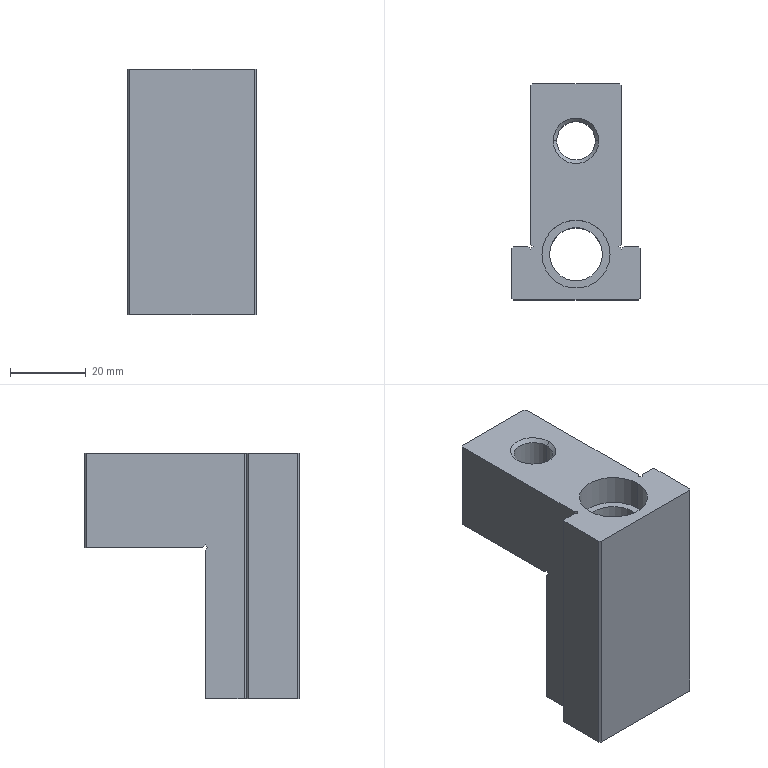Part | SolidWorks | features ICE 3, 3DProfileFeature 2, HoleWzd 2, Extrusion 1 | 1 solid | 41 faces | box 34 x 57 x 65 mm | volume 53450 mm3 | plane 29 | cylinder 8 | cone 4 | commonest cylinder face diameters 18 x4 10.2 x2 14 x2
STEP:
#1=CARTESIAN_POINT('',(-5.1,42.,64.075));
#2=VERTEX_POINT('',#1);
#3=CARTESIAN_POINT('',(5.1,42.,64.075));
#4=VERTEX_POINT('',#3);
#5=CARTESIAN_POINT('',(0.,42.,64.075));
#6=DIRECTION('',(0.,0.,1.));
#7=DIRECTION('',(1.,0.,0.));
#8=AXIS2_PLACEMENT_3D('',#5,#6,#7);
#9=CIRCLE('',#8,5.1);
#10=EDGE_CURVE('',#2,#4,#9,.T.);
#11=ORIENTED_EDGE('',*,*,#10,.F.);
#12=CARTESIAN_POINT('',(-6.025,42.,65.));
#13=VERTEX_POINT('',#12);
#14=CARTESIAN_POINT('',(-6.025,42.,65.));
#15=DIRECTION('',(-0.7071,0.,0.7071));
#16=VECTOR('',#15,1000.);
#17=LINE('',#14,#16);
#18=EDGE_CURVE('',#2,#13,#17,.T.);
#19=ORIENTED_EDGE('',*,*,#18,.T.);
#20=CARTESIAN_POINT('',(6.025,42.,65.));
#21=VERTEX_POINT('',#20);
#22=CARTESIAN_POINT('',(0.,42.,65.));
#23=DIRECTION('',(0.,0.,1.));
#24=DIRECTION('',(1.,0.,0.));
#25=AXIS2_PLACEMENT_3D('',#22,#23,#24);
#26=CIRCLE('',#25,6.025);
#27=EDGE_CURVE('',#13,#21,#26,.T.);
#28=ORIENTED_EDGE('',*,*,#27,.T.);
#29=CARTESIAN_POINT('',(6.025,42.,65.));
#30=DIRECTION('',(0.7071,0.,0.7071));
#31=VECTOR('',#30,1000.);
#32=LINE('',#29,#31);
#33=EDGE_CURVE('',#4,#21,#32,.T.);
#34=ORIENTED_EDGE('',*,*,#33,.F.);
#35=EDGE_LOOP('',(#11,#19,#28,#34));
#36=FACE_OUTER_BOUND('',#35,.T.);
#37=CARTESIAN_POINT('',(0.,42.,65.));
#38=DIRECTION('',(0.,0.,1.));
#39=DIRECTION('',(1.,0.,0.));
#40=AXIS2_PLACEMENT_3D('',#37,#38,#39);
#41=CONICAL_SURFACE('',#40,6.025,0.7854);
#42=ADVANCED_FACE('',(#36),#41,.F.);
#43=CARTESIAN_POINT('',(-5.1,42.,40.));
#44=VERTEX_POINT('',#43);
#45=CARTESIAN_POINT('',(5.1,42.,40.));
#46=VERTEX_POINT('',#45);
#47=CARTESIAN_POINT('',(0.,42.,40.));
#48=DIRECTION('',(0.,0.,1.));
#49=DIRECTION('',(0.,-1.,0.));
#50=AXIS2_PLACEMENT_3D('',#47,#48,#49);
#51=CIRCLE('',#50,5.1);
#52=EDGE_CURVE('',#44,#46,#51,.T.);
#53=ORIENTED_EDGE('',*,*,#52,.F.);
#54=CARTESIAN_POINT('',(-5.1,42.,65.));
#55=DIRECTION('',(0.,0.,1.));
#56=VECTOR('',#55,1000.);
#57=LINE('',#54,#56);
#58=EDGE_CURVE('',#44,#2,#57,.T.);
#59=ORIENTED_EDGE('',*,*,#58,.T.);
#60=ORIENTED_EDGE('',*,*,#10,.T.);
#61=CARTESIAN_POINT('',(5.1,42.,65.));
#62=DIRECTION('',(0.,0.,1.));
#63=VECTOR('',#62,1000.);
#64=LINE('',#61,#63);
#65=EDGE_CURVE('',#46,#4,#64,.T.);
#66=ORIENTED_EDGE('',*,*,#65,.F.);
#67=EDGE_LOOP('',(#53,#59,#60,#66));
#68=FACE_OUTER_BOUND('',#67,.T.);
#69=CARTESIAN_POINT('',(0.,42.,65.));
#70=DIRECTION('',(0.,0.,1.));
#71=DIRECTION('',(1.,0.,0.));
#72=AXIS2_PLACEMENT_3D('',#69,#70,#71);
#73=CYLINDRICAL_SURFACE('',#72,5.1);
#74=ADVANCED_FACE('',(#68),#73,.F.);
#75=CARTESIAN_POINT('',(7.,12.,9.025));
#76=VERTEX_POINT('',#75);
#77=CARTESIAN_POINT('',(-7.,12.,9.025));
#78=VERTEX_POINT('',#77);
#79=CARTESIAN_POINT('',(0.,12.,9.025));
#80=DIRECTION('',(0.,0.,-1.));
#81=DIRECTION('',(-1.,0.,0.));
#82=AXIS2_PLACEMENT_3D('',#79,#80,#81);
#83=CIRCLE('',#82,7.);
#84=EDGE_CURVE('',#76,#78,#83,.T.);
#85=ORIENTED_EDGE('',*,*,#84,.F.);
#86=CARTESIAN_POINT('',(8.025,12.,8.));
#87=VERTEX_POINT('',#86);
#88=CARTESIAN_POINT('',(8.025,12.,8.));
#89=DIRECTION('',(0.7071,0.,-0.7071));
#90=VECTOR('',#89,1000.);
#91=LINE('',#88,#90);
#92=EDGE_CURVE('',#76,#87,#91,.T.);
#93=ORIENTED_EDGE('',*,*,#92,.T.);
#94=CARTESIAN_POINT('',(-8.025,12.,8.));
#95=VERTEX_POINT('',#94);
#96=CARTESIAN_POINT('',(0.,12.,8.));
#97=DIRECTION('',(0.,0.,-1.));
#98=DIRECTION('',(-1.,0.,0.));
#99=AXIS2_PLACEMENT_3D('',#96,#97,#98);
#100=CIRCLE('',#99,8.025);
#101=EDGE_CURVE('',#87,#95,#100,.T.);
#102=ORIENTED_EDGE('',*,*,#101,.T.);
#103=CARTESIAN_POINT('',(-8.025,12.,8.));
#104=DIRECTION('',(-0.7071,0.,-0.7071));
#105=VECTOR('',#104,1000.);
#106=LINE('',#103,#105);
#107=EDGE_CURVE('',#78,#95,#106,.T.);
#108=ORIENTED_EDGE('',*,*,#107,.F.);
#109=EDGE_LOOP('',(#85,#93,#102,#108));
#110=FACE_OUTER_BOUND('',#109,.T.);
#111=CARTESIAN_POINT('',(0.,12.,8.));
#112=DIRECTION('',(0.,0.,-1.));
#113=DIRECTION('',(-1.,0.,0.));
#114=AXIS2_PLACEMENT_3D('',#111,#112,#113);
#115=CONICAL_SURFACE('',#114,8.025,0.7854);
#116=ADVANCED_FACE('',(#110),#115,.F.);
#117=CARTESIAN_POINT('',(-7.,12.,57.));
#118=VERTEX_POINT('',#117);
#119=CARTESIAN_POINT('',(7.,12.,57.));
#120=VERTEX_POINT('',#119);
#121=CARTESIAN_POINT('',(0.,12.,57.));
#122=DIRECTION('',(0.,0.,1.));
#123=DIRECTION('',(1.,0.,0.));
#124=AXIS2_PLACEMENT_3D('',#121,#122,#123);
#125=CIRCLE('',#124,7.);
#126=EDGE_CURVE('',#118,#120,#125,.T.);
#127=ORIENTED_EDGE('',*,*,#126,.T.);
#128=CARTESIAN_POINT('',(7.,12.,8.));
#129=DIRECTION('',(0.,0.,-1.));
#130=VECTOR('',#129,1000.);
#131=LINE('',#128,#130);
#132=EDGE_CURVE('',#120,#76,#131,.T.);
#133=ORIENTED_EDGE('',*,*,#132,.T.);
#134=ORIENTED_EDGE('',*,*,#84,.T.);
#135=CARTESIAN_POINT('',(-7.,12.,8.));
#136=DIRECTION('',(0.,0.,-1.));
#137=VECTOR('',#136,1000.);
#138=LINE('',#135,#137);
#139=EDGE_CURVE('',#118,#78,#138,.T.);
#140=ORIENTED_EDGE('',*,*,#139,.F.);
#141=EDGE_LOOP('',(#127,#133,#134,#140));
#142=FACE_OUTER_BOUND('',#141,.T.);
#143=CARTESIAN_POINT('',(0.,12.,8.));
#144=DIRECTION('',(0.,0.,-1.));
#145=DIRECTION('',(-1.,0.,0.));
#146=AXIS2_PLACEMENT_3D('',#143,#144,#145);
#147=CYLINDRICAL_SURFACE('',#146,7.);
#148=ADVANCED_FACE('',(#142),#147,.F.);
#149=CARTESIAN_POINT('',(9.,12.,8.));
#150=VERTEX_POINT('',#149);
#151=CARTESIAN_POINT('',(-9.,12.,8.));
#152=VERTEX_POINT('',#151);
#153=CARTESIAN_POINT('',(0.,12.,8.));
#154=DIRECTION('',(0.,0.,-1.));
#155=DIRECTION('',(-1.,0.,0.));
#156=AXIS2_PLACEMENT_3D('',#153,#154,#155);
#157=CIRCLE('',#156,9.);
#158=EDGE_CURVE('',#150,#152,#157,.T.);
#159=ORIENTED_EDGE('',*,*,#158,.F.);
#160=CARTESIAN_POINT('',(9.,12.,0.));
#161=VERTEX_POINT('',#160);
#162=CARTESIAN_POINT('',(9.,12.,8.));
#163=DIRECTION('',(0.,0.,-1.));
#164=VECTOR('',#163,1000.);
#165=LINE('',#162,#164);
#166=EDGE_CURVE('',#150,#161,#165,.T.);
#167=ORIENTED_EDGE('',*,*,#166,.T.);
#168=CARTESIAN_POINT('',(-9.,12.,0.));
#169=VERTEX_POINT('',#168);
#170=CARTESIAN_POINT('',(0.,12.,0.));
#171=DIRECTION('',(0.,0.,-1.));
#172=DIRECTION('',(-1.,0.,0.));
#173=AXIS2_PLACEMENT_3D('',#170,#171,#172);
#174=CIRCLE('',#173,9.);
#175=EDGE_CURVE('',#161,#169,#174,.T.);
#176=ORIENTED_EDGE('',*,*,#175,.T.);
#177=CARTESIAN_POINT('',(-9.,12.,8.));
#178=DIRECTION('',(0.,0.,-1.));
#179=VECTOR('',#178,1000.);
#180=LINE('',#177,#179);
#181=EDGE_CURVE('',#152,#169,#180,.T.);
#182=ORIENTED_EDGE('',*,*,#181,.F.);
#183=EDGE_LOOP('',(#159,#167,#176,#182));
#184=FACE_OUTER_BOUND('',#183,.T.);
#185=CARTESIAN_POINT('',(0.,12.,8.));
#186=DIRECTION('',(0.,0.,-1.));
#187=DIRECTION('',(-1.,0.,0.));
#188=AXIS2_PLACEMENT_3D('',#185,#186,#187);
#189=CYLINDRICAL_SURFACE('',#188,9.);
#190=ADVANCED_FACE('',(#184),#189,.F.);
#191=CARTESIAN_POINT('',(-9.,12.,57.));
#192=VERTEX_POINT('',#191);
#193=CARTESIAN_POINT('',(9.,12.,57.));
#194=VERTEX_POINT('',#193);
#195=CARTESIAN_POINT('',(0.,12.,57.));
#196=DIRECTION('',(0.,0.,1.));
#197=DIRECTION('',(1.,0.,0.));
#198=AXIS2_PLACEMENT_3D('',#195,#196,#197);
#199=CIRCLE('',#198,9.);
#200=EDGE_CURVE('',#192,#194,#199,.T.);
#201=ORIENTED_EDGE('',*,*,#200,.F.);
#202=CARTESIAN_POINT('',(-9.,12.,65.));
#203=VERTEX_POINT('',#202);
#204=CARTESIAN_POINT('',(-9.,12.,57.));
#205=DIRECTION('',(0.,0.,1.));
#206=VECTOR('',#205,1000.);
#207=LINE('',#204,#206);
#208=EDGE_CURVE('',#192,#203,#207,.T.);
#209=ORIENTED_EDGE('',*,*,#208,.T.);
#210=CARTESIAN_POINT('',(9.,12.,65.));
#211=VERTEX_POINT('',#210);
#212=CARTESIAN_POINT('',(0.,12.,65.));
#213=DIRECTION('',(0.,0.,1.));
#214=DIRECTION('',(1.,0.,0.));
#215=AXIS2_PLACEMENT_3D('',#212,#213,#214);
#216=CIRCLE('',#215,9.);
#217=EDGE_CURVE('',#203,#211,#216,.T.);
#218=ORIENTED_EDGE('',*,*,#217,.T.);
#219=CARTESIAN_POINT('',(9.,12.,57.));
#220=DIRECTION('',(0.,0.,1.));
#221=VECTOR('',#220,1000.);
#222=LINE('',#219,#221);
#223=EDGE_CURVE('',#194,#211,#222,.T.);
#224=ORIENTED_EDGE('',*,*,#223,.F.);
#225=EDGE_LOOP('',(#201,#209,#218,#224));
#226=FACE_OUTER_BOUND('',#225,.T.);
#227=CARTESIAN_POINT('',(0.,12.,57.));
#228=DIRECTION('',(0.,0.,1.));
#229=DIRECTION('',(1.,0.,0.));
#230=AXIS2_PLACEMENT_3D('',#227,#228,#229);
#231=CYLINDRICAL_SURFACE('',#230,9.);
#232=ADVANCED_FACE('',(#226),#231,.F.);
#233=CARTESIAN_POINT('',(-11.5,57.,65.));
#234=VERTEX_POINT('',#233);
#235=CARTESIAN_POINT('',(-11.5,57.,40.));
#236=VERTEX_POINT('',#235);
#237=CARTESIAN_POINT('',(-11.5,57.,65.));
#238=DIRECTION('',(0.,0.,-1.));
#239=VECTOR('',#238,1000.);
#240=LINE('',#237,#239);
#241=EDGE_CURVE('',#234,#236,#240,.T.);
#242=ORIENTED_EDGE('',*,*,#241,.T.);
#243=CARTESIAN_POINT('',(-12.,56.5,40.));
#244=VERTEX_POINT('',#243);
#245=CARTESIAN_POINT('',(-12.,56.5,40.));
#246=DIRECTION('',(-0.7071,-0.7071,0.));
#247=VECTOR('',#246,1000.);
#248=LINE('',#245,#247);
#249=EDGE_CURVE('',#236,#244,#248,.T.);
#250=ORIENTED_EDGE('',*,*,#249,.T.);
#251=CARTESIAN_POINT('',(-12.,56.5,65.));
#252=VERTEX_POINT('',#251);
#253=CARTESIAN_POINT('',(-12.,56.5,65.));
#254=DIRECTION('',(0.,0.,-1.));
#255=VECTOR('',#254,1000.);
#256=LINE('',#253,#255);
#257=EDGE_CURVE('',#252,#244,#256,.T.);
#258=ORIENTED_EDGE('',*,*,#257,.F.);
#259=CARTESIAN_POINT('',(-12.,56.5,65.));
#260=DIRECTION('',(-0.7071,-0.7071,0.));
#261=VECTOR('',#260,1000.);
#262=LINE('',#259,#261);
#263=EDGE_CURVE('',#234,#252,#262,.T.);
#264=ORIENTED_EDGE('',*,*,#263,.F.);
#265=EDGE_LOOP('',(#242,#250,#258,#264));
#266=FACE_OUTER_BOUND('',#265,.T.);
#267=CARTESIAN_POINT('',(-12.,56.5,65.));
#268=DIRECTION('',(0.7071,-0.7071,0.));
#269=DIRECTION('',(0.7071,0.7071,0.));
#270=AXIS2_PLACEMENT_3D('',#267,#268,#269);
#271=PLANE('',#270);
#272=ADVANCED_FACE('',(#266),#271,.F.);
#273=ORIENTED_EDGE('',*,*,#257,.T.);
#274=CARTESIAN_POINT('',(-12.,25.707,40.));
#275=VERTEX_POINT('',#274);
#276=CARTESIAN_POINT('',(-12.,14.707,40.));
#277=DIRECTION('',(0.,-1.,0.));
#278=VECTOR('',#277,1000.);
#279=LINE('',#276,#278);
#280=EDGE_CURVE('',#244,#275,#279,.T.);
#281=ORIENTED_EDGE('',*,*,#280,.T.);
#282=CARTESIAN_POINT('',(-12.,25.,40.707));
#283=VERTEX_POINT('',#282);
#284=CARTESIAN_POINT('',(-12.,7.707,58.));
#285=DIRECTION('',(0.,-0.7071,0.7071));
#286=VECTOR('',#285,1000.);
#287=LINE('',#284,#286);
#288=EDGE_CURVE('',#275,#283,#287,.T.);
#289=ORIENTED_EDGE('',*,*,#288,.T.);
#290=CARTESIAN_POINT('',(-12.,24.293,40.));
#291=VERTEX_POINT('',#290);
#292=CARTESIAN_POINT('',(-12.,32.,47.707));
#293=DIRECTION('',(0.,-0.7071,-0.7071));
#294=VECTOR('',#293,1000.);
#295=LINE('',#292,#294);
#296=EDGE_CURVE('',#283,#291,#295,.T.);
#297=ORIENTED_EDGE('',*,*,#296,.T.);
#298=CARTESIAN_POINT('',(-12.,25.,39.293));
#299=VERTEX_POINT('',#298);
#300=CARTESIAN_POINT('',(-12.,7.,57.293));
#301=DIRECTION('',(0.,0.7071,-0.7071));
#302=VECTOR('',#301,1000.);
#303=LINE('',#300,#302);
#304=EDGE_CURVE('',#291,#299,#303,.T.);
#305=ORIENTED_EDGE('',*,*,#304,.T.);
#306=CARTESIAN_POINT('',(-12.,25.,0.));
#307=VERTEX_POINT('',#306);
#308=CARTESIAN_POINT('',(-12.,25.,65.));
#309=DIRECTION('',(0.,0.,-1.));
#310=VECTOR('',#309,1000.);
#311=LINE('',#308,#310);
#312=EDGE_CURVE('',#299,#307,#311,.T.);
#313=ORIENTED_EDGE('',*,*,#312,.T.);
#314=CARTESIAN_POINT('',(-12.,14.707,0.));
#315=VERTEX_POINT('',#314);
#316=CARTESIAN_POINT('',(-12.,14.707,0.));
#317=DIRECTION('',(0.,-1.,0.));
#318=VECTOR('',#317,1000.);
#319=LINE('',#316,#318);
#320=EDGE_CURVE('',#307,#315,#319,.T.);
#321=ORIENTED_EDGE('',*,*,#320,.T.);
#322=CARTESIAN_POINT('',(-12.,14.707,65.));
#323=VERTEX_POINT('',#322);
#324=CARTESIAN_POINT('',(-12.,14.707,65.));
#325=DIRECTION('',(0.,0.,-1.));
#326=VECTOR('',#325,1000.);
#327=LINE('',#324,#326);
#328=EDGE_CURVE('',#323,#315,#327,.T.);
#329=ORIENTED_EDGE('',*,*,#328,.F.);
#330=CARTESIAN_POINT('',(-12.,14.707,65.));
#331=DIRECTION('',(0.,-1.,0.));
#332=VECTOR('',#331,1000.);
#333=LINE('',#330,#332);
#334=EDGE_CURVE('',#252,#323,#333,.T.);
#335=ORIENTED_EDGE('',*,*,#334,.F.);
#336=EDGE_LOOP('',(#273,#281,#289,#297,#305,#313,#321,#329,#335));
#337=FACE_OUTER_BOUND('',#336,.T.);
#338=CARTESIAN_POINT('',(-12.,14.707,65.));
#339=DIRECTION('',(1.,0.,0.));
#340=DIRECTION('',(0.,0.,-1.));
#341=AXIS2_PLACEMENT_3D('',#338,#339,#340);
#342=PLANE('',#341);
#343=ADVANCED_FACE('',(#337),#342,.F.);
#344=CARTESIAN_POINT('',(-11.293,14.,0.));
#345=VERTEX_POINT('',#344);
#346=CARTESIAN_POINT('',(-12.,14.707,0.));
#347=DIRECTION('',(0.7071,-0.7071,0.));
#348=VECTOR('',#347,1000.);
#349=LINE('',#346,#348);
#350=EDGE_CURVE('',#315,#345,#349,.T.);
#351=ORIENTED_EDGE('',*,*,#350,.T.);
#352=CARTESIAN_POINT('',(-11.293,14.,65.));
#353=VERTEX_POINT('',#352);
#354=CARTESIAN_POINT('',(-11.293,14.,65.));
#355=DIRECTION('',(0.,0.,-1.));
#356=VECTOR('',#355,1000.);
#357=LINE('',#354,#356);
#358=EDGE_CURVE('',#353,#345,#357,.T.);
#359=ORIENTED_EDGE('',*,*,#358,.F.);
#360=CARTESIAN_POINT('',(-12.,14.707,65.));
#361=DIRECTION('',(0.7071,-0.7071,0.));
#362=VECTOR('',#361,1000.);
#363=LINE('',#360,#362);
#364=EDGE_CURVE('',#323,#353,#363,.T.);
#365=ORIENTED_EDGE('',*,*,#364,.F.);
#366=ORIENTED_EDGE('',*,*,#328,.T.);
#367=EDGE_LOOP('',(#351,#359,#365,#366));
#368=FACE_OUTER_BOUND('',#367,.T.);
#369=CARTESIAN_POINT('',(-12.,14.707,65.));
#370=DIRECTION('',(0.7071,0.7071,0.));
#371=DIRECTION('',(-0.7071,0.7071,0.));
#372=AXIS2_PLACEMENT_3D('',#369,#370,#371);
#373=PLANE('',#372);
#374=ADVANCED_FACE('',(#368),#373,.F.);
#375=CARTESIAN_POINT('',(-12.,13.293,0.));
#376=VERTEX_POINT('',#375);
#377=CARTESIAN_POINT('',(-12.,13.293,0.));
#378=DIRECTION('',(-0.7071,-0.7071,0.));
#379=VECTOR('',#378,1000.);
#380=LINE('',#377,#379);
#381=EDGE_CURVE('',#345,#376,#380,.T.);
#382=ORIENTED_EDGE('',*,*,#381,.T.);
#383=CARTESIAN_POINT('',(-12.,13.293,65.));
#384=VERTEX_POINT('',#383);
#385=CARTESIAN_POINT('',(-12.,13.293,65.));
#386=DIRECTION('',(0.,0.,-1.));
#387=VECTOR('',#386,1000.);
#388=LINE('',#385,#387);
#389=EDGE_CURVE('',#384,#376,#388,.T.);
#390=ORIENTED_EDGE('',*,*,#389,.F.);
#391=CARTESIAN_POINT('',(-12.,13.293,65.));
#392=DIRECTION('',(-0.7071,-0.7071,0.));
#393=VECTOR('',#392,1000.);
#394=LINE('',#391,#393);
#395=EDGE_CURVE('',#353,#384,#394,.T.);
#396=ORIENTED_EDGE('',*,*,#395,.F.);
#397=ORIENTED_EDGE('',*,*,#358,.T.);
#398=EDGE_LOOP('',(#382,#390,#396,#397));
#399=FACE_OUTER_BOUND('',#398,.T.);
#400=CARTESIAN_POINT('',(-12.,13.293,65.));
#401=DIRECTION('',(0.7071,-0.7071,0.));
#402=DIRECTION('',(0.7071,0.7071,0.));
#403=AXIS2_PLACEMENT_3D('',#400,#401,#402);
#404=PLANE('',#403);
#405=ADVANCED_FACE('',(#399),#404,.F.);
#406=CARTESIAN_POINT('',(-12.707,14.,0.));
#407=VERTEX_POINT('',#406);
#408=CARTESIAN_POINT('',(-12.707,14.,0.));
#409=DIRECTION('',(-0.7071,0.7071,0.));
#410=VECTOR('',#409,1000.);
#411=LINE('',#408,#410);
#412=EDGE_CURVE('',#376,#407,#411,.T.);
#413=ORIENTED_EDGE('',*,*,#412,.T.);
#414=CARTESIAN_POINT('',(-12.707,14.,65.));
#415=VERTEX_POINT('',#414);
#416=CARTESIAN_POINT('',(-12.707,14.,65.));
#417=DIRECTION('',(0.,0.,-1.));
#418=VECTOR('',#417,1000.);
#419=LINE('',#416,#418);
#420=EDGE_CURVE('',#415,#407,#419,.T.);
#421=ORIENTED_EDGE('',*,*,#420,.F.);
#422=CARTESIAN_POINT('',(-12.707,14.,65.));
#423=DIRECTION('',(-0.7071,0.7071,0.));
#424=VECTOR('',#423,1000.);
#425=LINE('',#422,#424);
#426=EDGE_CURVE('',#384,#415,#425,.T.);
#427=ORIENTED_EDGE('',*,*,#426,.F.);
#428=ORIENTED_EDGE('',*,*,#389,.T.);
#429=EDGE_LOOP('',(#413,#421,#427,#428));
#430=FACE_OUTER_BOUND('',#429,.T.);
#431=CARTESIAN_POINT('',(-12.707,14.,65.));
#432=DIRECTION('',(-0.7071,-0.7071,0.));
#433=DIRECTION('',(0.7071,-0.7071,0.));
#434=AXIS2_PLACEMENT_3D('',#431,#432,#433);
#435=PLANE('',#434);
#436=ADVANCED_FACE('',(#430),#435,.F.);
#437=CARTESIAN_POINT('',(-16.5,14.,0.));
#438=VERTEX_POINT('',#437);
#439=CARTESIAN_POINT('',(-16.5,14.,0.));
#440=DIRECTION('',(-1.,0.,0.));
#441=VECTOR('',#440,1000.);
#442=LINE('',#439,#441);
#443=EDGE_CURVE('',#407,#438,#442,.T.);
#444=ORIENTED_EDGE('',*,*,#443,.T.);
#445=CARTESIAN_POINT('',(-16.5,14.,65.));
#446=VERTEX_POINT('',#445);
#447=CARTESIAN_POINT('',(-16.5,14.,65.));
#448=DIRECTION('',(0.,0.,-1.));
#449=VECTOR('',#448,1000.);
#450=LINE('',#447,#449);
#451=EDGE_CURVE('',#446,#438,#450,.T.);
#452=ORIENTED_EDGE('',*,*,#451,.F.);
#453=CARTESIAN_POINT('',(-16.5,14.,65.));
#454=DIRECTION('',(-1.,0.,0.));
#455=VECTOR('',#454,1000.);
#456=LINE('',#453,#455);
#457=EDGE_CURVE('',#415,#446,#456,.T.);
#458=ORIENTED_EDGE('',*,*,#457,.F.);
#459=ORIENTED_EDGE('',*,*,#420,.T.);
#460=EDGE_LOOP('',(#444,#452,#458,#459));
#461=FACE_OUTER_BOUND('',#460,.T.);
#462=CARTESIAN_POINT('',(-16.5,14.,65.));
#463=DIRECTION('',(0.,-1.,0.));
#464=DIRECTION('',(1.,0.,0.));
#465=AXIS2_PLACEMENT_3D('',#462,#463,#464);
#466=PLANE('',#465);
#467=ADVANCED_FACE('',(#461),#466,.F.);
#468=CARTESIAN_POINT('',(-17.,13.5,0.));
#469=VERTEX_POINT('',#468);
#470=CARTESIAN_POINT('',(-17.,13.5,0.));
#471=DIRECTION('',(-0.7071,-0.7071,0.));
#472=VECTOR('',#471,1000.);
#473=LINE('',#470,#472);
#474=EDGE_CURVE('',#438,#469,#473,.T.);
#475=ORIENTED_EDGE('',*,*,#474,.T.);
#476=CARTESIAN_POINT('',(-17.,13.5,65.));
#477=VERTEX_POINT('',#476);
#478=CARTESIAN_POINT('',(-17.,13.5,65.));
#479=DIRECTION('',(0.,0.,-1.));
#480=VECTOR('',#479,1000.);
#481=LINE('',#478,#480);
#482=EDGE_CURVE('',#477,#469,#481,.T.);
#483=ORIENTED_EDGE('',*,*,#482,.F.);
#484=CARTESIAN_POINT('',(-17.,13.5,65.));
#485=DIRECTION('',(-0.7071,-0.7071,0.));
#486=VECTOR('',#485,1000.);
#487=LINE('',#484,#486);
#488=EDGE_CURVE('',#446,#477,#487,.T.);
#489=ORIENTED_EDGE('',*,*,#488,.F.);
#490=ORIENTED_EDGE('',*,*,#451,.T.);
#491=EDGE_LOOP('',(#475,#483,#489,#490));
#492=FACE_OUTER_BOUND('',#491,.T.);
#493=CARTESIAN_POINT('',(-17.,13.5,65.));
#494=DIRECTION('',(0.7071,-0.7071,0.));
#495=DIRECTION('',(0.7071,0.7071,0.));
#496=AXIS2_PLACEMENT_3D('',#493,#494,#495);
#497=PLANE('',#496);
#498=ADVANCED_FACE('',(#492),#497,.F.);
#499=CARTESIAN_POINT('',(-17.,0.5,0.));
#500=VERTEX_POINT('',#499);
#501=CARTESIAN_POINT('',(-17.,0.5,0.));
#502=DIRECTION('',(0.,-1.,0.));
#503=VECTOR('',#502,1000.);
#504=LINE('',#501,#503);
#505=EDGE_CURVE('',#469,#500,#504,.T.);
#506=ORIENTED_EDGE('',*,*,#505,.T.);
#507=CARTESIAN_POINT('',(-17.,0.5,65.));
#508=VERTEX_POINT('',#507);
#509=CARTESIAN_POINT('',(-17.,0.5,65.));
#510=DIRECTION('',(0.,0.,-1.));
#511=VECTOR('',#510,1000.);
#512=LINE('',#509,#511);
#513=EDGE_CURVE('',#508,#500,#512,.T.);
#514=ORIENTED_EDGE('',*,*,#513,.F.);
#515=CARTESIAN_POINT('',(-17.,0.5,65.));
#516=DIRECTION('',(0.,-1.,0.));
#517=VECTOR('',#516,1000.);
#518=LINE('',#515,#517);
#519=EDGE_CURVE('',#477,#508,#518,.T.);
#520=ORIENTED_EDGE('',*,*,#519,.F.);
#521=ORIENTED_EDGE('',*,*,#482,.T.);
#522=EDGE_LOOP('',(#506,#514,#520,#521));
#523=FACE_OUTER_BOUND('',#522,.T.);
#524=CARTESIAN_POINT('',(-17.,0.5,65.));
#525=DIRECTION('',(1.,0.,0.));
#526=DIRECTION('',(0.,0.,-1.));
#527=AXIS2_PLACEMENT_3D('',#524,#525,#526);
#528=PLANE('',#527);
#529=ADVANCED_FACE('',(#523),#528,.F.);
#530=CARTESIAN_POINT('',(-16.5,0.,0.));
#531=VERTEX_POINT('',#530);
#532=CARTESIAN_POINT('',(-16.5,0.,0.));
#533=DIRECTION('',(0.7071,-0.7071,0.));
#534=VECTOR('',#533,1000.);
#535=LINE('',#532,#534);
#536=EDGE_CURVE('',#500,#531,#535,.T.);
#537=ORIENTED_EDGE('',*,*,#536,.T.);
#538=CARTESIAN_POINT('',(-16.5,0.,65.));
#539=VERTEX_POINT('',#538);
#540=CARTESIAN_POINT('',(-16.5,0.,65.));
#541=DIRECTION('',(0.,0.,-1.));
#542=VECTOR('',#541,1000.);
#543=LINE('',#540,#542);
#544=EDGE_CURVE('',#539,#531,#543,.T.);
#545=ORIENTED_EDGE('',*,*,#544,.F.);
#546=CARTESIAN_POINT('',(-16.5,0.,65.));
#547=DIRECTION('',(0.7071,-0.7071,0.));
#548=VECTOR('',#547,1000.);
#549=LINE('',#546,#548);
#550=EDGE_CURVE('',#508,#539,#549,.T.);
#551=ORIENTED_EDGE('',*,*,#550,.F.);
#552=ORIENTED_EDGE('',*,*,#513,.T.);
#553=EDGE_LOOP('',(#537,#545,#551,#552));
#554=FACE_OUTER_BOUND('',#553,.T.);
#555=CARTESIAN_POINT('',(-16.5,0.,65.));
#556=DIRECTION('',(0.7071,0.7071,0.));
#557=DIRECTION('',(-0.7071,0.7071,0.));
#558=AXIS2_PLACEMENT_3D('',#555,#556,#557);
#559=PLANE('',#558);
#560=ADVANCED_FACE('',(#554),#559,.F.);
#561=CARTESIAN_POINT('',(16.5,0.,0.));
#562=VERTEX_POINT('',#561);
#563=CARTESIAN_POINT('',(16.5,0.,0.));
#564=DIRECTION('',(1.,0.,0.));
#565=VECTOR('',#564,1000.);
#566=LINE('',#563,#565);
#567=EDGE_CURVE('',#531,#562,#566,.T.);
#568=ORIENTED_EDGE('',*,*,#567,.T.);
#569=CARTESIAN_POINT('',(16.5,0.,65.));
#570=VERTEX_POINT('',#569);
#571=CARTESIAN_POINT('',(16.5,0.,65.));
#572=DIRECTION('',(0.,0.,-1.));
#573=VECTOR('',#572,1000.);
#574=LINE('',#571,#573);
#575=EDGE_CURVE('',#570,#562,#574,.T.);
#576=ORIENTED_EDGE('',*,*,#575,.F.);
#577=CARTESIAN_POINT('',(16.5,0.,65.));
#578=DIRECTION('',(1.,0.,0.));
#579=VECTOR('',#578,1000.);
#580=LINE('',#577,#579);
#581=EDGE_CURVE('',#539,#570,#580,.T.);
#582=ORIENTED_EDGE('',*,*,#581,.F.);
#583=ORIENTED_EDGE('',*,*,#544,.T.);
#584=EDGE_LOOP('',(#568,#576,#582,#583));
#585=FACE_OUTER_BOUND('',#584,.T.);
#586=CARTESIAN_POINT('',(16.5,0.,65.));
#587=DIRECTION('',(0.,1.,0.));
#588=DIRECTION('',(0.,0.,1.));
#589=AXIS2_PLACEMENT_3D('',#586,#587,#588);
#590=PLANE('',#589);
#591=ADVANCED_FACE('',(#585),#590,.F.);
#592=CARTESIAN_POINT('',(17.,0.5,0.));
#593=VERTEX_POINT('',#592);
#594=CARTESIAN_POINT('',(16.5,0.,0.));
#595=DIRECTION('',(0.7071,0.7071,0.));
#596=VECTOR('',#595,1000.);
#597=LINE('',#594,#596);
#598=EDGE_CURVE('',#562,#593,#597,.T.);
#599=ORIENTED_EDGE('',*,*,#598,.T.);
#600=CARTESIAN_POINT('',(17.,0.5,65.));
#601=VERTEX_POINT('',#600);
#602=CARTESIAN_POINT('',(17.,0.5,65.));
#603=DIRECTION('',(0.,0.,-1.));
#604=VECTOR('',#603,1000.);
#605=LINE('',#602,#604);
#606=EDGE_CURVE('',#601,#593,#605,.T.);
#607=ORIENTED_EDGE('',*,*,#606,.F.);
#608=CARTESIAN_POINT('',(16.5,0.,65.));
#609=DIRECTION('',(0.7071,0.7071,0.));
#610=VECTOR('',#609,1000.);
#611=LINE('',#608,#610);
#612=EDGE_CURVE('',#570,#601,#611,.T.);
#613=ORIENTED_EDGE('',*,*,#612,.F.);
#614=ORIENTED_EDGE('',*,*,#575,.T.);
#615=EDGE_LOOP('',(#599,#607,#613,#614));
#616=FACE_OUTER_BOUND('',#615,.T.);
#617=CARTESIAN_POINT('',(16.5,0.,65.));
#618=DIRECTION('',(-0.7071,0.7071,0.));
#619=DIRECTION('',(-0.7071,-0.7071,0.));
#620=AXIS2_PLACEMENT_3D('',#617,#618,#619);
#621=PLANE('',#620);
#622=ADVANCED_FACE('',(#616),#621,.F.);
#623=CARTESIAN_POINT('',(17.,13.5,0.));
#624=VERTEX_POINT('',#623);
#625=CARTESIAN_POINT('',(17.,0.5,0.));
#626=DIRECTION('',(0.,1.,0.));
#627=VECTOR('',#626,1000.);
#628=LINE('',#625,#627);
#629=EDGE_CURVE('',#593,#624,#628,.T.);
#630=ORIENTED_EDGE('',*,*,#629,.T.);
#631=CARTESIAN_POINT('',(17.,13.5,65.));
#632=VERTEX_POINT('',#631);
#633=CARTESIAN_POINT('',(17.,13.5,65.));
#634=DIRECTION('',(0.,0.,-1.));
#635=VECTOR('',#634,1000.);
#636=LINE('',#633,#635);
#637=EDGE_CURVE('',#632,#624,#636,.T.);
#638=ORIENTED_EDGE('',*,*,#637,.F.);
#639=CARTESIAN_POINT('',(17.,0.5,65.));
#640=DIRECTION('',(0.,1.,0.));
#641=VECTOR('',#640,1000.);
#642=LINE('',#639,#641);
#643=EDGE_CURVE('',#601,#632,#642,.T.);
#644=ORIENTED_EDGE('',*,*,#643,.F.);
#645=ORIENTED_EDGE('',*,*,#606,.T.);
#646=EDGE_LOOP('',(#630,#638,#644,#645));
#647=FACE_OUTER_BOUND('',#646,.T.);
#648=CARTESIAN_POINT('',(17.,0.5,65.));
#649=DIRECTION('',(-1.,0.,0.));
#650=DIRECTION('',(0.,0.,1.));
#651=AXIS2_PLACEMENT_3D('',#648,#649,#650);
#652=PLANE('',#651);
#653=ADVANCED_FACE('',(#647),#652,.F.);
#654=CARTESIAN_POINT('',(16.5,14.,0.));
#655=VERTEX_POINT('',#654);
#656=CARTESIAN_POINT('',(17.,13.5,0.));
#657=DIRECTION('',(-0.7071,0.7071,0.));
#658=VECTOR('',#657,1000.);
#659=LINE('',#656,#658);
#660=EDGE_CURVE('',#624,#655,#659,.T.);
#661=ORIENTED_EDGE('',*,*,#660,.T.);
#662=CARTESIAN_POINT('',(16.5,14.,65.));
#663=VERTEX_POINT('',#662);
#664=CARTESIAN_POINT('',(16.5,14.,65.));
#665=DIRECTION('',(0.,0.,-1.));
#666=VECTOR('',#665,1000.);
#667=LINE('',#664,#666);
#668=EDGE_CURVE('',#663,#655,#667,.T.);
#669=ORIENTED_EDGE('',*,*,#668,.F.);
#670=CARTESIAN_POINT('',(17.,13.5,65.));
#671=DIRECTION('',(-0.7071,0.7071,0.));
#672=VECTOR('',#671,1000.);
#673=LINE('',#670,#672);
#674=EDGE_CURVE('',#632,#663,#673,.T.);
#675=ORIENTED_EDGE('',*,*,#674,.F.);
#676=ORIENTED_EDGE('',*,*,#637,.T.);
#677=EDGE_LOOP('',(#661,#669,#675,#676));
#678=FACE_OUTER_BOUND('',#677,.T.);
#679=CARTESIAN_POINT('',(17.,13.5,65.));
#680=DIRECTION('',(-0.7071,-0.7071,0.));
#681=DIRECTION('',(0.7071,-0.7071,0.));
#682=AXIS2_PLACEMENT_3D('',#679,#680,#681);
#683=PLANE('',#682);
#684=ADVANCED_FACE('',(#678),#683,.F.);
#685=CARTESIAN_POINT('',(12.707,14.,0.));
#686=VERTEX_POINT('',#685);
#687=CARTESIAN_POINT('',(16.5,14.,0.));
#688=DIRECTION('',(-1.,0.,0.));
#689=VECTOR('',#688,1000.);
#690=LINE('',#687,#689);
#691=EDGE_CURVE('',#655,#686,#690,.T.);
#692=ORIENTED_EDGE('',*,*,#691,.T.);
#693=CARTESIAN_POINT('',(12.707,14.,65.));
#694=VERTEX_POINT('',#693);
#695=CARTESIAN_POINT('',(12.707,14.,65.));
#696=DIRECTION('',(0.,0.,-1.));
#697=VECTOR('',#696,1000.);
#698=LINE('',#695,#697);
#699=EDGE_CURVE('',#694,#686,#698,.T.);
#700=ORIENTED_EDGE('',*,*,#699,.F.);
#701=CARTESIAN_POINT('',(16.5,14.,65.));
#702=DIRECTION('',(-1.,0.,0.));
#703=VECTOR('',#702,1000.);
#704=LINE('',#701,#703);
#705=EDGE_CURVE('',#663,#694,#704,.T.);
#706=ORIENTED_EDGE('',*,*,#705,.F.);
#707=ORIENTED_EDGE('',*,*,#668,.T.);
#708=EDGE_LOOP('',(#692,#700,#706,#707));
#709=FACE_OUTER_BOUND('',#708,.T.);
#710=CARTESIAN_POINT('',(16.5,14.,65.));
#711=DIRECTION('',(0.,-1.,0.));
#712=DIRECTION('',(1.,0.,0.));
#713=AXIS2_PLACEMENT_3D('',#710,#711,#712);
#714=PLANE('',#713);
#715=ADVANCED_FACE('',(#709),#714,.F.);
#716=CARTESIAN_POINT('',(12.,13.293,0.));
#717=VERTEX_POINT('',#716);
#718=CARTESIAN_POINT('',(12.707,14.,0.));
#719=DIRECTION('',(-0.7071,-0.7071,0.));
#720=VECTOR('',#719,1000.);
#721=LINE('',#718,#720);
#722=EDGE_CURVE('',#686,#717,#721,.T.);
#723=ORIENTED_EDGE('',*,*,#722,.T.);
#724=CARTESIAN_POINT('',(12.,13.293,65.));
#725=VERTEX_POINT('',#724);
#726=CARTESIAN_POINT('',(12.,13.293,65.));
#727=DIRECTION('',(0.,0.,-1.));
#728=VECTOR('',#727,1000.);
#729=LINE('',#726,#728);
#730=EDGE_CURVE('',#725,#717,#729,.T.);
#731=ORIENTED_EDGE('',*,*,#730,.F.);
#732=CARTESIAN_POINT('',(12.707,14.,65.));
#733=DIRECTION('',(-0.7071,-0.7071,0.));
#734=VECTOR('',#733,1000.);
#735=LINE('',#732,#734);
#736=EDGE_CURVE('',#694,#725,#735,.T.);
#737=ORIENTED_EDGE('',*,*,#736,.F.);
#738=ORIENTED_EDGE('',*,*,#699,.T.);
#739=EDGE_LOOP('',(#723,#731,#737,#738));
#740=FACE_OUTER_BOUND('',#739,.T.);
#741=CARTESIAN_POINT('',(12.707,14.,65.));
#742=DIRECTION('',(0.7071,-0.7071,0.));
#743=DIRECTION('',(0.7071,0.7071,0.));
#744=AXIS2_PLACEMENT_3D('',#741,#742,#743);
#745=PLANE('',#744);
#746=ADVANCED_FACE('',(#740),#745,.F.);
#747=CARTESIAN_POINT('',(11.293,14.,0.));
#748=VERTEX_POINT('',#747);
#749=CARTESIAN_POINT('',(12.,13.293,0.));
#750=DIRECTION('',(-0.7071,0.7071,0.));
#751=VECTOR('',#750,1000.);
#752=LINE('',#749,#751);
#753=EDGE_CURVE('',#717,#748,#752,.T.);
#754=ORIENTED_EDGE('',*,*,#753,.T.);
#755=CARTESIAN_POINT('',(11.293,14.,65.));
#756=VERTEX_POINT('',#755);
#757=CARTESIAN_POINT('',(11.293,14.,65.));
#758=DIRECTION('',(0.,0.,-1.));
#759=VECTOR('',#758,1000.);
#760=LINE('',#757,#759);
#761=EDGE_CURVE('',#756,#748,#760,.T.);
#762=ORIENTED_EDGE('',*,*,#761,.F.);
#763=CARTESIAN_POINT('',(12.,13.293,65.));
#764=DIRECTION('',(-0.7071,0.7071,0.));
#765=VECTOR('',#764,1000.);
#766=LINE('',#763,#765);
#767=EDGE_CURVE('',#725,#756,#766,.T.);
#768=ORIENTED_EDGE('',*,*,#767,.F.);
#769=ORIENTED_EDGE('',*,*,#730,.T.);
#770=EDGE_LOOP('',(#754,#762,#768,#769));
#771=FACE_OUTER_BOUND('',#770,.T.);
#772=CARTESIAN_POINT('',(12.,13.293,65.));
#773=DIRECTION('',(-0.7071,-0.7071,0.));
#774=DIRECTION('',(0.7071,-0.7071,0.));
#775=AXIS2_PLACEMENT_3D('',#772,#773,#774);
#776=PLANE('',#775);
#777=ADVANCED_FACE('',(#771),#776,.F.);
#778=CARTESIAN_POINT('',(12.,14.707,0.));
#779=VERTEX_POINT('',#778);
#780=CARTESIAN_POINT('',(12.,14.707,0.));
#781=DIRECTION('',(0.7071,0.7071,0.));
#782=VECTOR('',#781,1000.);
#783=LINE('',#780,#782);
#784=EDGE_CURVE('',#748,#779,#783,.T.);
#785=ORIENTED_EDGE('',*,*,#784,.T.);
#786=CARTESIAN_POINT('',(12.,14.707,65.));
#787=VERTEX_POINT('',#786);
#788=CARTESIAN_POINT('',(12.,14.707,65.));
#789=DIRECTION('',(0.,0.,-1.));
#790=VECTOR('',#789,1000.);
#791=LINE('',#788,#790);
#792=EDGE_CURVE('',#787,#779,#791,.T.);
#793=ORIENTED_EDGE('',*,*,#792,.F.);
#794=CARTESIAN_POINT('',(12.,14.707,65.));
#795=DIRECTION('',(0.7071,0.7071,0.));
#796=VECTOR('',#795,1000.);
#797=LINE('',#794,#796);
#798=EDGE_CURVE('',#756,#787,#797,.T.);
#799=ORIENTED_EDGE('',*,*,#798,.F.);
#800=ORIENTED_EDGE('',*,*,#761,.T.);
#801=EDGE_LOOP('',(#785,#793,#799,#800));
#802=FACE_OUTER_BOUND('',#801,.T.);
#803=CARTESIAN_POINT('',(12.,14.707,65.));
#804=DIRECTION('',(-0.7071,0.7071,0.));
#805=DIRECTION('',(-0.7071,-0.7071,0.));
#806=AXIS2_PLACEMENT_3D('',#803,#804,#805);
#807=PLANE('',#806);
#808=ADVANCED_FACE('',(#802),#807,.F.);
#809=CARTESIAN_POINT('',(12.,25.,40.707));
#810=VERTEX_POINT('',#809);
#811=CARTESIAN_POINT('',(12.,25.707,40.));
#812=VERTEX_POINT('',#811);
#813=CARTESIAN_POINT('',(12.,7.707,58.));
#814=DIRECTION('',(0.,0.7071,-0.7071));
#815=VECTOR('',#814,1000.);
#816=LINE('',#813,#815);
#817=EDGE_CURVE('',#810,#812,#816,.T.);
#818=ORIENTED_EDGE('',*,*,#817,.T.);
#819=CARTESIAN_POINT('',(12.,56.5,40.));
#820=VERTEX_POINT('',#819);
#821=CARTESIAN_POINT('',(12.,14.707,40.));
#822=DIRECTION('',(0.,1.,0.));
#823=VECTOR('',#822,1000.);
#824=LINE('',#821,#823);
#825=EDGE_CURVE('',#812,#820,#824,.T.);
#826=ORIENTED_EDGE('',*,*,#825,.T.);
#827=CARTESIAN_POINT('',(12.,56.5,65.));
#828=VERTEX_POINT('',#827);
#829=CARTESIAN_POINT('',(12.,56.5,65.));
#830=DIRECTION('',(0.,0.,-1.));
#831=VECTOR('',#830,1000.);
#832=LINE('',#829,#831);
#833=EDGE_CURVE('',#828,#820,#832,.T.);
#834=ORIENTED_EDGE('',*,*,#833,.F.);
#835=CARTESIAN_POINT('',(12.,14.707,65.));
#836=DIRECTION('',(0.,1.,0.));
#837=VECTOR('',#836,1000.);
#838=LINE('',#835,#837);
#839=EDGE_CURVE('',#787,#828,#838,.T.);
#840=ORIENTED_EDGE('',*,*,#839,.F.);
#841=ORIENTED_EDGE('',*,*,#792,.T.);
#842=CARTESIAN_POINT('',(12.,25.,0.));
#843=VERTEX_POINT('',#842);
#844=CARTESIAN_POINT('',(12.,14.707,0.));
#845=DIRECTION('',(0.,1.,0.));
#846=VECTOR('',#845,1000.);
#847=LINE('',#844,#846);
#848=EDGE_CURVE('',#779,#843,#847,.T.);
#849=ORIENTED_EDGE('',*,*,#848,.T.);
#850=CARTESIAN_POINT('',(12.,25.,39.293));
#851=VERTEX_POINT('',#850);
#852=CARTESIAN_POINT('',(12.,25.,65.));
#853=DIRECTION('',(0.,0.,1.));
#854=VECTOR('',#853,1000.);
#855=LINE('',#852,#854);
#856=EDGE_CURVE('',#843,#851,#855,.T.);
#857=ORIENTED_EDGE('',*,*,#856,.T.);
#858=CARTESIAN_POINT('',(12.,24.293,40.));
#859=VERTEX_POINT('',#858);
#860=CARTESIAN_POINT('',(12.,7.,57.293));
#861=DIRECTION('',(0.,-0.7071,0.7071));
#862=VECTOR('',#861,1000.);
#863=LINE('',#860,#862);
#864=EDGE_CURVE('',#851,#859,#863,.T.);
#865=ORIENTED_EDGE('',*,*,#864,.T.);
#866=CARTESIAN_POINT('',(12.,32.,47.707));
#867=DIRECTION('',(0.,0.7071,0.7071));
#868=VECTOR('',#867,1000.);
#869=LINE('',#866,#868);
#870=EDGE_CURVE('',#859,#810,#869,.T.);
#871=ORIENTED_EDGE('',*,*,#870,.T.);
#872=EDGE_LOOP('',(#818,#826,#834,#840,#841,#849,#857,#865,#871));
#873=FACE_OUTER_BOUND('',#872,.T.);
#874=CARTESIAN_POINT('',(12.,14.707,65.));
#875=DIRECTION('',(-1.,0.,0.));
#876=DIRECTION('',(0.,0.,1.));
#877=AXIS2_PLACEMENT_3D('',#874,#875,#876);
#878=PLANE('',#877);
#879=ADVANCED_FACE('',(#873),#878,.F.);
#880=ORIENTED_EDGE('',*,*,#833,.T.);
#881=CARTESIAN_POINT('',(11.5,57.,40.));
#882=VERTEX_POINT('',#881);
#883=CARTESIAN_POINT('',(12.,56.5,40.));
#884=DIRECTION('',(-0.7071,0.7071,0.));
#885=VECTOR('',#884,1000.);
#886=LINE('',#883,#885);
#887=EDGE_CURVE('',#820,#882,#886,.T.);
#888=ORIENTED_EDGE('',*,*,#887,.T.);
#889=CARTESIAN_POINT('',(11.5,57.,65.));
#890=VERTEX_POINT('',#889);
#891=CARTESIAN_POINT('',(11.5,57.,65.));
#892=DIRECTION('',(0.,0.,-1.));
#893=VECTOR('',#892,1000.);
#894=LINE('',#891,#893);
#895=EDGE_CURVE('',#890,#882,#894,.T.);
#896=ORIENTED_EDGE('',*,*,#895,.F.);
#897=CARTESIAN_POINT('',(12.,56.5,65.));
#898=DIRECTION('',(-0.7071,0.7071,0.));
#899=VECTOR('',#898,1000.);
#900=LINE('',#897,#899);
#901=EDGE_CURVE('',#828,#890,#900,.T.);
#902=ORIENTED_EDGE('',*,*,#901,.F.);
#903=EDGE_LOOP('',(#880,#888,#896,#902));
#904=FACE_OUTER_BOUND('',#903,.T.);
#905=CARTESIAN_POINT('',(12.,56.5,65.));
#906=DIRECTION('',(-0.7071,-0.7071,0.));
#907=DIRECTION('',(0.7071,-0.7071,0.));
#908=AXIS2_PLACEMENT_3D('',#905,#906,#907);
#909=PLANE('',#908);
#910=ADVANCED_FACE('',(#904),#909,.F.);
#911=ORIENTED_EDGE('',*,*,#895,.T.);
#912=CARTESIAN_POINT('',(-11.5,57.,40.));
#913=DIRECTION('',(-1.,0.,0.));
#914=VECTOR('',#913,1000.);
#915=LINE('',#912,#914);
#916=EDGE_CURVE('',#882,#236,#915,.T.);
#917=ORIENTED_EDGE('',*,*,#916,.T.);
#918=ORIENTED_EDGE('',*,*,#241,.F.);
#919=CARTESIAN_POINT('',(-11.5,57.,65.));
#920=DIRECTION('',(-1.,0.,0.));
#921=VECTOR('',#920,1000.);
#922=LINE('',#919,#921);
#923=EDGE_CURVE('',#890,#234,#922,.T.);
#924=ORIENTED_EDGE('',*,*,#923,.F.);
#925=EDGE_LOOP('',(#911,#917,#918,#924));
#926=FACE_OUTER_BOUND('',#925,.T.);
#927=CARTESIAN_POINT('',(-11.5,57.,65.));
#928=DIRECTION('',(0.,-1.,0.));
#929=DIRECTION('',(0.,0.,-1.));
#930=AXIS2_PLACEMENT_3D('',#927,#928,#929);
#931=PLANE('',#930);
#932=ADVANCED_FACE('',(#926),#931,.F.);
#933=CARTESIAN_POINT('',(0.,42.,65.));
#934=DIRECTION('',(0.,0.,1.));
#935=DIRECTION('',(1.,0.,0.));
#936=AXIS2_PLACEMENT_3D('',#933,#934,#935);
#937=CIRCLE('',#936,6.025);
#938=EDGE_CURVE('',#21,#13,#937,.T.);
#939=ORIENTED_EDGE('',*,*,#938,.F.);
#940=ORIENTED_EDGE('',*,*,#27,.F.);
#941=EDGE_LOOP('',(#939,#940));
#942=FACE_BOUND('',#941,.T.);
#943=CARTESIAN_POINT('',(0.,12.,65.));
#944=DIRECTION('',(0.,0.,1.));
#945=DIRECTION('',(1.,0.,0.));
#946=AXIS2_PLACEMENT_3D('',#943,#944,#945);
#947=CIRCLE('',#946,9.);
#948=EDGE_CURVE('',#211,#203,#947,.T.);
#949=ORIENTED_EDGE('',*,*,#948,.F.);
#950=ORIENTED_EDGE('',*,*,#217,.F.);
#951=EDGE_LOOP('',(#949,#950));
#952=FACE_BOUND('',#951,.T.);
#953=ORIENTED_EDGE('',*,*,#263,.T.);
#954=ORIENTED_EDGE('',*,*,#334,.T.);
#955=ORIENTED_EDGE('',*,*,#364,.T.);
#956=ORIENTED_EDGE('',*,*,#395,.T.);
#957=ORIENTED_EDGE('',*,*,#426,.T.);
#958=ORIENTED_EDGE('',*,*,#457,.T.);
#959=ORIENTED_EDGE('',*,*,#488,.T.);
#960=ORIENTED_EDGE('',*,*,#519,.T.);
#961=ORIENTED_EDGE('',*,*,#550,.T.);
#962=ORIENTED_EDGE('',*,*,#581,.T.);
#963=ORIENTED_EDGE('',*,*,#612,.T.);
#964=ORIENTED_EDGE('',*,*,#643,.T.);
#965=ORIENTED_EDGE('',*,*,#674,.T.);
#966=ORIENTED_EDGE('',*,*,#705,.T.);
#967=ORIENTED_EDGE('',*,*,#736,.T.);
#968=ORIENTED_EDGE('',*,*,#767,.T.);
#969=ORIENTED_EDGE('',*,*,#798,.T.);
#970=ORIENTED_EDGE('',*,*,#839,.T.);
#971=ORIENTED_EDGE('',*,*,#901,.T.);
#972=ORIENTED_EDGE('',*,*,#923,.T.);
#973=EDGE_LOOP('',(#953,#954,#955,#956,#957,#958,#959,#960,#961,#962,#963,#964,#965,#966,#967,#968,#969,#970,#971,#972));
#974=FACE_OUTER_BOUND('',#973,.T.);
#975=CARTESIAN_POINT('',(0.,0.,65.));
#976=DIRECTION('',(0.,0.,1.));
#977=DIRECTION('',(1.,0.,0.));
#978=AXIS2_PLACEMENT_3D('',#975,#976,#977);
#979=PLANE('',#978);
#980=ADVANCED_FACE('',(#942,#952,#974),#979,.T.);
#981=CARTESIAN_POINT('',(0.,12.,0.));
#982=DIRECTION('',(0.,0.,-1.));
#983=DIRECTION('',(-1.,0.,0.));
#984=AXIS2_PLACEMENT_3D('',#981,#982,#983);
#985=CIRCLE('',#984,9.);
#986=EDGE_CURVE('',#169,#161,#985,.T.);
#987=ORIENTED_EDGE('',*,*,#986,.F.);
#988=ORIENTED_EDGE('',*,*,#175,.F.);
#989=EDGE_LOOP('',(#987,#988));
#990=FACE_BOUND('',#989,.T.);
#991=ORIENTED_EDGE('',*,*,#320,.F.);
#992=CARTESIAN_POINT('',(0.,25.,0.));
#993=DIRECTION('',(1.,0.,0.));
#994=VECTOR('',#993,1000.);
#995=LINE('',#992,#994);
#996=EDGE_CURVE('',#307,#843,#995,.T.);
#997=ORIENTED_EDGE('',*,*,#996,.T.);
#998=ORIENTED_EDGE('',*,*,#848,.F.);
#999=ORIENTED_EDGE('',*,*,#784,.F.);
#1000=ORIENTED_EDGE('',*,*,#753,.F.);
#1001=ORIENTED_EDGE('',*,*,#722,.F.);
#1002=ORIENTED_EDGE('',*,*,#691,.F.);
#1003=ORIENTED_EDGE('',*,*,#660,.F.);
#1004=ORIENTED_EDGE('',*,*,#629,.F.);
#1005=ORIENTED_EDGE('',*,*,#598,.F.);
#1006=ORIENTED_EDGE('',*,*,#567,.F.);
#1007=ORIENTED_EDGE('',*,*,#536,.F.);
#1008=ORIENTED_EDGE('',*,*,#505,.F.);
#1009=ORIENTED_EDGE('',*,*,#474,.F.);
#1010=ORIENTED_EDGE('',*,*,#443,.F.);
#1011=ORIENTED_EDGE('',*,*,#412,.F.);
#1012=ORIENTED_EDGE('',*,*,#381,.F.);
#1013=ORIENTED_EDGE('',*,*,#350,.F.);
#1014=EDGE_LOOP('',(#991,#997,#998,#999,#1000,#1001,#1002,#1003,#1004,#1005,#1006,#1007,#1008,#1009,#1010,#1011,#1012,#1013));
#1015=FACE_OUTER_BOUND('',#1014,.T.);
#1016=CARTESIAN_POINT('',(0.,0.,0.));
#1017=DIRECTION('',(0.,0.,1.));
#1018=DIRECTION('',(1.,0.,0.));
#1019=AXIS2_PLACEMENT_3D('',#1016,#1017,#1018);
#1020=PLANE('',#1019);
#1021=ADVANCED_FACE('',(#990,#1015),#1020,.F.);
#1022=CARTESIAN_POINT('',(-17.,24.293,40.));
#1023=DIRECTION('',(1.,0.,0.));
#1024=VECTOR('',#1023,1000.);
#1025=LINE('',#1022,#1024);
#1026=EDGE_CURVE('',#291,#859,#1025,.T.);
#1027=ORIENTED_EDGE('',*,*,#1026,.T.);
#1028=ORIENTED_EDGE('',*,*,#864,.F.);
#1029=CARTESIAN_POINT('',(-17.,25.,39.293));
#1030=DIRECTION('',(1.,0.,0.));
#1031=VECTOR('',#1030,1000.);
#1032=LINE('',#1029,#1031);
#1033=EDGE_CURVE('',#299,#851,#1032,.T.);
#1034=ORIENTED_EDGE('',*,*,#1033,.F.);
#1035=ORIENTED_EDGE('',*,*,#304,.F.);
#1036=EDGE_LOOP('',(#1027,#1028,#1034,#1035));
#1037=FACE_OUTER_BOUND('',#1036,.T.);
#1038=CARTESIAN_POINT('',(-17.,24.293,40.));
#1039=DIRECTION('',(0.,-0.7071,-0.7071));
#1040=DIRECTION('',(0.,0.7071,-0.7071));
#1041=AXIS2_PLACEMENT_3D('',#1038,#1039,#1040);
#1042=PLANE('',#1041);
#1043=ADVANCED_FACE('',(#1037),#1042,.F.);
#1044=CARTESIAN_POINT('',(-17.,25.,40.707));
#1045=DIRECTION('',(1.,0.,0.));
#1046=VECTOR('',#1045,1000.);
#1047=LINE('',#1044,#1046);
#1048=EDGE_CURVE('',#283,#810,#1047,.T.);
#1049=ORIENTED_EDGE('',*,*,#1048,.T.);
#1050=ORIENTED_EDGE('',*,*,#870,.F.);
#1051=ORIENTED_EDGE('',*,*,#1026,.F.);
#1052=ORIENTED_EDGE('',*,*,#296,.F.);
#1053=EDGE_LOOP('',(#1049,#1050,#1051,#1052));
#1054=FACE_OUTER_BOUND('',#1053,.T.);
#1055=CARTESIAN_POINT('',(-17.,25.,40.707));
#1056=DIRECTION('',(0.,-0.7071,0.7071));
#1057=DIRECTION('',(0.,-0.7071,-0.7071));
#1058=AXIS2_PLACEMENT_3D('',#1055,#1056,#1057);
#1059=PLANE('',#1058);
#1060=ADVANCED_FACE('',(#1054),#1059,.F.);
#1061=CARTESIAN_POINT('',(-17.,25.707,40.));
#1062=DIRECTION('',(1.,0.,0.));
#1063=VECTOR('',#1062,1000.);
#1064=LINE('',#1061,#1063);
#1065=EDGE_CURVE('',#275,#812,#1064,.T.);
#1066=ORIENTED_EDGE('',*,*,#1065,.T.);
#1067=ORIENTED_EDGE('',*,*,#817,.F.);
#1068=ORIENTED_EDGE('',*,*,#1048,.F.);
#1069=ORIENTED_EDGE('',*,*,#288,.F.);
#1070=EDGE_LOOP('',(#1066,#1067,#1068,#1069));
#1071=FACE_OUTER_BOUND('',#1070,.T.);
#1072=CARTESIAN_POINT('',(-17.,25.707,40.));
#1073=DIRECTION('',(0.,0.7071,0.7071));
#1074=DIRECTION('',(0.,-0.7071,0.7071));
#1075=AXIS2_PLACEMENT_3D('',#1072,#1073,#1074);
#1076=PLANE('',#1075);
#1077=ADVANCED_FACE('',(#1071),#1076,.F.);
#1078=CARTESIAN_POINT('',(0.,42.,40.));
#1079=DIRECTION('',(0.,0.,1.));
#1080=DIRECTION('',(0.,-1.,0.));
#1081=AXIS2_PLACEMENT_3D('',#1078,#1079,#1080);
#1082=CIRCLE('',#1081,5.1);
#1083=EDGE_CURVE('',#46,#44,#1082,.T.);
#1084=ORIENTED_EDGE('',*,*,#1083,.T.);
#1085=ORIENTED_EDGE('',*,*,#52,.T.);
#1086=EDGE_LOOP('',(#1084,#1085));
#1087=FACE_BOUND('',#1086,.T.);
#1088=ORIENTED_EDGE('',*,*,#249,.F.);
#1089=ORIENTED_EDGE('',*,*,#916,.F.);
#1090=ORIENTED_EDGE('',*,*,#887,.F.);
#1091=ORIENTED_EDGE('',*,*,#825,.F.);
#1092=ORIENTED_EDGE('',*,*,#1065,.F.);
#1093=ORIENTED_EDGE('',*,*,#280,.F.);
#1094=EDGE_LOOP('',(#1088,#1089,#1090,#1091,#1092,#1093));
#1095=FACE_OUTER_BOUND('',#1094,.T.);
#1096=CARTESIAN_POINT('',(-17.,79.715,40.));
#1097=DIRECTION('',(0.,0.,1.));
#1098=DIRECTION('',(0.,-1.,0.));
#1099=AXIS2_PLACEMENT_3D('',#1096,#1097,#1098);
#1100=PLANE('',#1099);
#1101=ADVANCED_FACE('',(#1087,#1095),#1100,.F.);
#1102=ORIENTED_EDGE('',*,*,#1033,.T.);
#1103=ORIENTED_EDGE('',*,*,#856,.F.);
#1104=ORIENTED_EDGE('',*,*,#996,.F.);
#1105=ORIENTED_EDGE('',*,*,#312,.F.);
#1106=EDGE_LOOP('',(#1102,#1103,#1104,#1105));
#1107=FACE_OUTER_BOUND('',#1106,.T.);
#1108=CARTESIAN_POINT('',(-17.,25.,39.293));
#1109=DIRECTION('',(0.,-1.,0.));
#1110=DIRECTION('',(0.,0.,-1.));
#1111=AXIS2_PLACEMENT_3D('',#1108,#1109,#1110);
#1112=PLANE('',#1111);
#1113=ADVANCED_FACE('',(#1107),#1112,.F.);
#1114=ORIENTED_EDGE('',*,*,#208,.F.);
#1115=CARTESIAN_POINT('',(0.,12.,57.));
#1116=DIRECTION('',(0.,0.,1.));
#1117=DIRECTION('',(1.,0.,0.));
#1118=AXIS2_PLACEMENT_3D('',#1115,#1116,#1117);
#1119=CIRCLE('',#1118,9.);
#1120=EDGE_CURVE('',#194,#192,#1119,.T.);
#1121=ORIENTED_EDGE('',*,*,#1120,.F.);
#1122=ORIENTED_EDGE('',*,*,#223,.T.);
#1123=ORIENTED_EDGE('',*,*,#948,.T.);
#1124=EDGE_LOOP('',(#1114,#1121,#1122,#1123));
#1125=FACE_OUTER_BOUND('',#1124,.T.);
#1126=CARTESIAN_POINT('',(0.,12.,57.));
#1127=DIRECTION('',(0.,0.,1.));
#1128=DIRECTION('',(1.,0.,0.));
#1129=AXIS2_PLACEMENT_3D('',#1126,#1127,#1128);
#1130=CYLINDRICAL_SURFACE('',#1129,9.);
#1131=ADVANCED_FACE('',(#1125),#1130,.F.);
#1132=ORIENTED_EDGE('',*,*,#126,.F.);
#1133=CARTESIAN_POINT('',(0.,12.,57.));
#1134=DIRECTION('',(0.,0.,1.));
#1135=DIRECTION('',(1.,0.,0.));
#1136=AXIS2_PLACEMENT_3D('',#1133,#1134,#1135);
#1137=CIRCLE('',#1136,7.);
#1138=EDGE_CURVE('',#120,#118,#1137,.T.);
#1139=ORIENTED_EDGE('',*,*,#1138,.F.);
#1140=EDGE_LOOP('',(#1132,#1139));
#1141=FACE_BOUND('',#1140,.T.);
#1142=ORIENTED_EDGE('',*,*,#1120,.T.);
#1143=ORIENTED_EDGE('',*,*,#200,.T.);
#1144=EDGE_LOOP('',(#1142,#1143));
#1145=FACE_OUTER_BOUND('',#1144,.T.);
#1146=CARTESIAN_POINT('',(0.,12.,57.));
#1147=DIRECTION('',(0.,0.,1.));
#1148=DIRECTION('',(1.,0.,0.));
#1149=AXIS2_PLACEMENT_3D('',#1146,#1147,#1148);
#1150=PLANE('',#1149);
#1151=ADVANCED_FACE('',(#1141,#1145),#1150,.T.);
#1152=ORIENTED_EDGE('',*,*,#166,.F.);
#1153=CARTESIAN_POINT('',(0.,12.,8.));
#1154=DIRECTION('',(0.,0.,-1.));
#1155=DIRECTION('',(-1.,0.,0.));
#1156=AXIS2_PLACEMENT_3D('',#1153,#1154,#1155);
#1157=CIRCLE('',#1156,9.);
#1158=EDGE_CURVE('',#152,#150,#1157,.T.);
#1159=ORIENTED_EDGE('',*,*,#1158,.F.);
#1160=ORIENTED_EDGE('',*,*,#181,.T.);
#1161=ORIENTED_EDGE('',*,*,#986,.T.);
#1162=EDGE_LOOP('',(#1152,#1159,#1160,#1161));
#1163=FACE_OUTER_BOUND('',#1162,.T.);
#1164=CARTESIAN_POINT('',(0.,12.,8.));
#1165=DIRECTION('',(0.,0.,-1.));
#1166=DIRECTION('',(-1.,0.,0.));
#1167=AXIS2_PLACEMENT_3D('',#1164,#1165,#1166);
#1168=CYLINDRICAL_SURFACE('',#1167,9.);
#1169=ADVANCED_FACE('',(#1163),#1168,.F.);
#1170=CARTESIAN_POINT('',(0.,12.,8.));
#1171=DIRECTION('',(0.,0.,-1.));
#1172=DIRECTION('',(-1.,0.,0.));
#1173=AXIS2_PLACEMENT_3D('',#1170,#1171,#1172);
#1174=CIRCLE('',#1173,8.025);
#1175=EDGE_CURVE('',#95,#87,#1174,.T.);
#1176=ORIENTED_EDGE('',*,*,#1175,.F.);
#1177=ORIENTED_EDGE('',*,*,#101,.F.);
#1178=EDGE_LOOP('',(#1176,#1177));
#1179=FACE_BOUND('',#1178,.T.);
#1180=ORIENTED_EDGE('',*,*,#1158,.T.);
#1181=ORIENTED_EDGE('',*,*,#158,.T.);
#1182=EDGE_LOOP('',(#1180,#1181));
#1183=FACE_OUTER_BOUND('',#1182,.T.);
#1184=CARTESIAN_POINT('',(0.,12.,8.));
#1185=DIRECTION('',(0.,0.,-1.));
#1186=DIRECTION('',(-1.,0.,0.));
#1187=AXIS2_PLACEMENT_3D('',#1184,#1185,#1186);
#1188=PLANE('',#1187);
#1189=ADVANCED_FACE('',(#1179,#1183),#1188,.T.);
#1190=ORIENTED_EDGE('',*,*,#132,.F.);
#1191=ORIENTED_EDGE('',*,*,#1138,.T.);
#1192=ORIENTED_EDGE('',*,*,#139,.T.);
#1193=CARTESIAN_POINT('',(0.,12.,9.025));
#1194=DIRECTION('',(0.,0.,-1.));
#1195=DIRECTION('',(-1.,0.,0.));
#1196=AXIS2_PLACEMENT_3D('',#1193,#1194,#1195);
#1197=CIRCLE('',#1196,7.);
#1198=EDGE_CURVE('',#78,#76,#1197,.T.);
#1199=ORIENTED_EDGE('',*,*,#1198,.T.);
#1200=EDGE_LOOP('',(#1190,#1191,#1192,#1199));
#1201=FACE_OUTER_BOUND('',#1200,.T.);
#1202=CARTESIAN_POINT('',(0.,12.,8.));
#1203=DIRECTION('',(0.,0.,-1.));
#1204=DIRECTION('',(-1.,0.,0.));
#1205=AXIS2_PLACEMENT_3D('',#1202,#1203,#1204);
#1206=CYLINDRICAL_SURFACE('',#1205,7.);
#1207=ADVANCED_FACE('',(#1201),#1206,.F.);
#1208=ORIENTED_EDGE('',*,*,#92,.F.);
#1209=ORIENTED_EDGE('',*,*,#1198,.F.);
#1210=ORIENTED_EDGE('',*,*,#107,.T.);
#1211=ORIENTED_EDGE('',*,*,#1175,.T.);
#1212=EDGE_LOOP('',(#1208,#1209,#1210,#1211));
#1213=FACE_OUTER_BOUND('',#1212,.T.);
#1214=CARTESIAN_POINT('',(0.,12.,8.));
#1215=DIRECTION('',(0.,0.,-1.));
#1216=DIRECTION('',(-1.,0.,0.));
#1217=AXIS2_PLACEMENT_3D('',#1214,#1215,#1216);
#1218=CONICAL_SURFACE('',#1217,8.025,0.7854);
#1219=ADVANCED_FACE('',(#1213),#1218,.F.);
#1220=ORIENTED_EDGE('',*,*,#58,.F.);
#1221=ORIENTED_EDGE('',*,*,#1083,.F.);
#1222=ORIENTED_EDGE('',*,*,#65,.T.);
#1223=CARTESIAN_POINT('',(0.,42.,64.075));
#1224=DIRECTION('',(0.,0.,1.));
#1225=DIRECTION('',(1.,0.,0.));
#1226=AXIS2_PLACEMENT_3D('',#1223,#1224,#1225);
#1227=CIRCLE('',#1226,5.1);
#1228=EDGE_CURVE('',#4,#2,#1227,.T.);
#1229=ORIENTED_EDGE('',*,*,#1228,.T.);
#1230=EDGE_LOOP('',(#1220,#1221,#1222,#1229));
#1231=FACE_OUTER_BOUND('',#1230,.T.);
#1232=CARTESIAN_POINT('',(0.,42.,65.));
#1233=DIRECTION('',(0.,0.,1.));
#1234=DIRECTION('',(1.,0.,0.));
#1235=AXIS2_PLACEMENT_3D('',#1232,#1233,#1234);
#1236=CYLINDRICAL_SURFACE('',#1235,5.1);
#1237=ADVANCED_FACE('',(#1231),#1236,.F.);
#1238=ORIENTED_EDGE('',*,*,#18,.F.);
#1239=ORIENTED_EDGE('',*,*,#1228,.F.);
#1240=ORIENTED_EDGE('',*,*,#33,.T.);
#1241=ORIENTED_EDGE('',*,*,#938,.T.);
#1242=EDGE_LOOP('',(#1238,#1239,#1240,#1241));
#1243=FACE_OUTER_BOUND('',#1242,.T.);
#1244=CARTESIAN_POINT('',(0.,42.,65.));
#1245=DIRECTION('',(0.,0.,1.));
#1246=DIRECTION('',(1.,0.,0.));
#1247=AXIS2_PLACEMENT_3D('',#1244,#1245,#1246);
#1248=CONICAL_SURFACE('',#1247,6.025,0.7854);
#1249=ADVANCED_FACE('',(#1243),#1248,.F.);
#1250=CLOSED_SHELL('',(#42,#74,#116,#148,#190,#232,#272,#343,#374,#405,#436,#467,#498,#529,#560,#591,#622,#653,#684,#715,#746,#777,#808,#879,#910,#932,#980,#1021,#1043,#1060,#1077,#1101,#1113,#1131,#1151,#1169,#1189,#1207,#1219,#1237,#1249));
#1251=MANIFOLD_SOLID_BREP('',#1250);
#1252=CARTESIAN_POINT('',(0.,0.,0.));
#1253=DIRECTION('',(0.,0.,1.));
#1254=DIRECTION('',(1.,0.,0.));
#1255=AXIS2_PLACEMENT_3D('',#1252,#1253,#1254);
#1256=(LENGTH_UNIT()NAMED_UNIT(*)SI_UNIT(.MILLI.,.METRE.));
#1257=UNCERTAINTY_MEASURE_WITH_UNIT(LENGTH_MEASURE(0.00001),#1256,'','');
#1258=(NAMED_UNIT(*)PLANE_ANGLE_UNIT()SI_UNIT($,.RADIAN.));
#1259=(NAMED_UNIT(*)SI_UNIT($,.STERADIAN.)SOLID_ANGLE_UNIT());
#1260=(GEOMETRIC_REPRESENTATION_CONTEXT(3)GLOBAL_UNCERTAINTY_ASSIGNED_CONTEXT((#1257))GLOBAL_UNIT_ASSIGNED_CONTEXT((#1256,#1258,#1259))REPRESENTATION_CONTEXT('',''));
#1261=ADVANCED_BREP_SHAPE_REPRESENTATION('',(#1251,#1255),#1260);